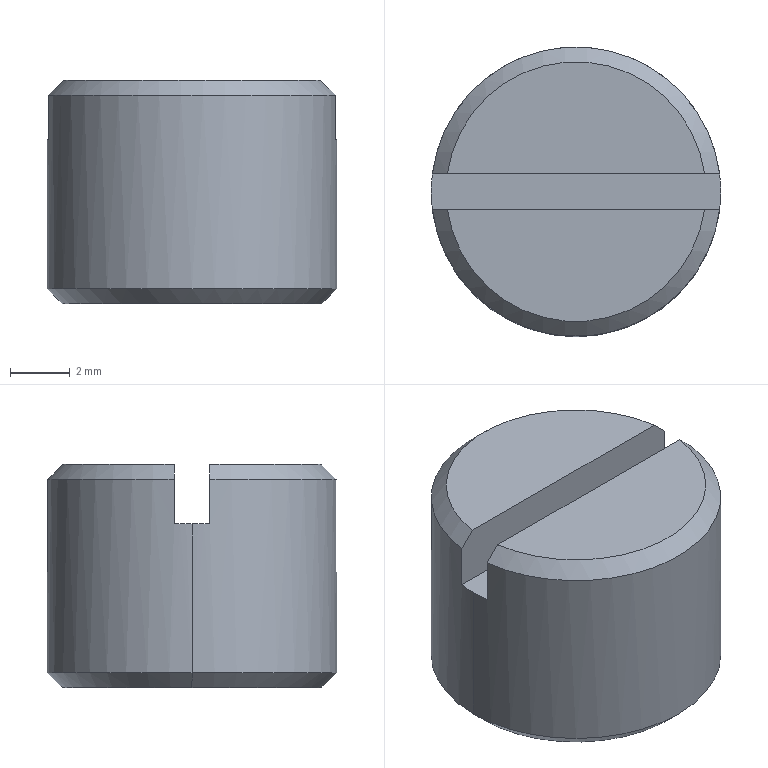Part | SolidWorks | features Chamfer 1, Extrusion 1, ICE 1 | 1 solid | 12 faces | box 9.73 x 9.73 x 7.5 mm | volume 527.297 mm3 | plane 6 | cone 4 | cylinder 2 | commonest cylinder face diameters 9.73 x2
STEP:
#1=CARTESIAN_POINT('',(-4.365,0.,0.));
#2=VERTEX_POINT('',#1);
#3=CARTESIAN_POINT('',(4.365,0.,0.));
#4=VERTEX_POINT('',#3);
#5=CARTESIAN_POINT('',(0.,0.,0.));
#6=DIRECTION('',(0.,0.,-1.));
#7=DIRECTION('',(1.,0.,0.));
#8=AXIS2_PLACEMENT_3D('',#5,#6,#7);
#9=CIRCLE('',#8,4.365);
#10=EDGE_CURVE('',#2,#4,#9,.T.);
#11=ORIENTED_EDGE('',*,*,#10,.F.);
#12=CARTESIAN_POINT('',(-4.865,0.,0.5));
#13=VERTEX_POINT('',#12);
#14=CARTESIAN_POINT('',(-4.865,0.,0.5));
#15=DIRECTION('',(-0.7071,0.,0.7071));
#16=VECTOR('',#15,1000.);
#17=LINE('',#14,#16);
#18=EDGE_CURVE('',#2,#13,#17,.T.);
#19=ORIENTED_EDGE('',*,*,#18,.T.);
#20=CARTESIAN_POINT('',(4.865,0.,0.5));
#21=VERTEX_POINT('',#20);
#22=CARTESIAN_POINT('',(0.,0.,0.5));
#23=DIRECTION('',(0.,0.,1.));
#24=DIRECTION('',(1.,0.,0.));
#25=AXIS2_PLACEMENT_3D('',#22,#23,#24);
#26=CIRCLE('',#25,4.865);
#27=EDGE_CURVE('',#21,#13,#26,.T.);
#28=ORIENTED_EDGE('',*,*,#27,.F.);
#29=CARTESIAN_POINT('',(4.865,0.,0.5));
#30=DIRECTION('',(0.7071,0.,0.7071));
#31=VECTOR('',#30,1000.);
#32=LINE('',#29,#31);
#33=EDGE_CURVE('',#4,#21,#32,.T.);
#34=ORIENTED_EDGE('',*,*,#33,.F.);
#35=EDGE_LOOP('',(#11,#19,#28,#34));
#36=FACE_OUTER_BOUND('',#35,.T.);
#37=CARTESIAN_POINT('',(0.,0.,0.5));
#38=DIRECTION('',(0.,0.,1.));
#39=DIRECTION('',(1.,0.,0.));
#40=AXIS2_PLACEMENT_3D('',#37,#38,#39);
#41=CONICAL_SURFACE('',#40,4.865,0.7854);
#42=ADVANCED_FACE('',(#36),#41,.T.);
#43=CARTESIAN_POINT('',(4.865,0.,5.5));
#44=VERTEX_POINT('',#43);
#45=CARTESIAN_POINT('',(4.828,0.6,5.5));
#46=VERTEX_POINT('',#45);
#47=CARTESIAN_POINT('',(0.,0.,5.5));
#48=DIRECTION('',(0.,0.,1.));
#49=DIRECTION('',(1.,0.,0.));
#50=AXIS2_PLACEMENT_3D('',#47,#48,#49);
#51=CIRCLE('',#50,4.865);
#52=EDGE_CURVE('',#44,#46,#51,.T.);
#53=ORIENTED_EDGE('',*,*,#52,.F.);
#54=CARTESIAN_POINT('',(4.865,0.,7.5));
#55=DIRECTION('',(0.,0.,-1.));
#56=VECTOR('',#55,1000.);
#57=LINE('',#54,#56);
#58=EDGE_CURVE('',#44,#21,#57,.T.);
#59=ORIENTED_EDGE('',*,*,#58,.T.);
#60=ORIENTED_EDGE('',*,*,#27,.T.);
#61=CARTESIAN_POINT('',(-4.865,0.,5.5));
#62=VERTEX_POINT('',#61);
#63=CARTESIAN_POINT('',(-4.865,0.,7.5));
#64=DIRECTION('',(0.,0.,-1.));
#65=VECTOR('',#64,1000.);
#66=LINE('',#63,#65);
#67=EDGE_CURVE('',#62,#13,#66,.T.);
#68=ORIENTED_EDGE('',*,*,#67,.F.);
#69=CARTESIAN_POINT('',(-4.828,0.6,5.5));
#70=VERTEX_POINT('',#69);
#71=CARTESIAN_POINT('',(0.,0.,5.5));
#72=DIRECTION('',(0.,0.,1.));
#73=DIRECTION('',(1.,0.,0.));
#74=AXIS2_PLACEMENT_3D('',#71,#72,#73);
#75=CIRCLE('',#74,4.865);
#76=EDGE_CURVE('',#70,#62,#75,.T.);
#77=ORIENTED_EDGE('',*,*,#76,.F.);
#78=CARTESIAN_POINT('',(-4.828,0.6,7.));
#79=VERTEX_POINT('',#78);
#80=CARTESIAN_POINT('',(-4.828,0.6,7.5));
#81=DIRECTION('',(0.,0.,1.));
#82=VECTOR('',#81,1000.);
#83=LINE('',#80,#82);
#84=EDGE_CURVE('',#70,#79,#83,.T.);
#85=ORIENTED_EDGE('',*,*,#84,.T.);
#86=CARTESIAN_POINT('',(4.828,0.6,7.));
#87=VERTEX_POINT('',#86);
#88=CARTESIAN_POINT('',(0.,0.,7.));
#89=DIRECTION('',(0.,0.,-1.));
#90=DIRECTION('',(1.,0.,0.));
#91=AXIS2_PLACEMENT_3D('',#88,#89,#90);
#92=CIRCLE('',#91,4.865);
#93=EDGE_CURVE('',#79,#87,#92,.T.);
#94=ORIENTED_EDGE('',*,*,#93,.T.);
#95=CARTESIAN_POINT('',(4.828,0.6,7.5));
#96=DIRECTION('',(0.,0.,-1.));
#97=VECTOR('',#96,1000.);
#98=LINE('',#95,#97);
#99=EDGE_CURVE('',#87,#46,#98,.T.);
#100=ORIENTED_EDGE('',*,*,#99,.T.);
#101=EDGE_LOOP('',(#53,#59,#60,#68,#77,#85,#94,#100));
#102=FACE_OUTER_BOUND('',#101,.T.);
#103=CARTESIAN_POINT('',(0.,0.,7.5));
#104=DIRECTION('',(0.,0.,-1.));
#105=DIRECTION('',(-1.,0.,0.));
#106=AXIS2_PLACEMENT_3D('',#103,#104,#105);
#107=CYLINDRICAL_SURFACE('',#106,4.865);
#108=ADVANCED_FACE('',(#102),#107,.T.);
#109=CARTESIAN_POINT('',(4.324,0.6,7.5));
#110=VERTEX_POINT('',#109);
#111=CARTESIAN_POINT('',(-4.324,0.6,7.5));
#112=VERTEX_POINT('',#111);
#113=CARTESIAN_POINT('',(0.,0.6,7.5));
#114=DIRECTION('',(-1.,0.,0.));
#115=VECTOR('',#114,1000.);
#116=LINE('',#113,#115);
#117=EDGE_CURVE('',#110,#112,#116,.T.);
#118=ORIENTED_EDGE('',*,*,#117,.F.);
#119=CARTESIAN_POINT('',(0.,0.,7.5));
#120=DIRECTION('',(0.,0.,1.));
#121=DIRECTION('',(1.,0.,0.));
#122=AXIS2_PLACEMENT_3D('',#119,#120,#121);
#123=CIRCLE('',#122,4.365);
#124=EDGE_CURVE('',#110,#112,#123,.T.);
#125=ORIENTED_EDGE('',*,*,#124,.T.);
#126=EDGE_LOOP('',(#118,#125));
#127=FACE_OUTER_BOUND('',#126,.T.);
#128=CARTESIAN_POINT('',(0.,0.,7.5));
#129=DIRECTION('',(0.,0.,1.));
#130=DIRECTION('',(1.,0.,0.));
#131=AXIS2_PLACEMENT_3D('',#128,#129,#130);
#132=PLANE('',#131);
#133=ADVANCED_FACE('',(#127),#132,.T.);
#134=ORIENTED_EDGE('',*,*,#58,.F.);
#135=CARTESIAN_POINT('',(4.828,-0.6,5.5));
#136=VERTEX_POINT('',#135);
#137=CARTESIAN_POINT('',(0.,0.,5.5));
#138=DIRECTION('',(0.,0.,1.));
#139=DIRECTION('',(1.,0.,0.));
#140=AXIS2_PLACEMENT_3D('',#137,#138,#139);
#141=CIRCLE('',#140,4.865);
#142=EDGE_CURVE('',#136,#44,#141,.T.);
#143=ORIENTED_EDGE('',*,*,#142,.F.);
#144=CARTESIAN_POINT('',(4.828,-0.6,7.));
#145=VERTEX_POINT('',#144);
#146=CARTESIAN_POINT('',(4.828,-0.6,7.5));
#147=DIRECTION('',(0.,0.,1.));
#148=VECTOR('',#147,1000.);
#149=LINE('',#146,#148);
#150=EDGE_CURVE('',#136,#145,#149,.T.);
#151=ORIENTED_EDGE('',*,*,#150,.T.);
#152=CARTESIAN_POINT('',(-4.828,-0.6,7.));
#153=VERTEX_POINT('',#152);
#154=CARTESIAN_POINT('',(0.,0.,7.));
#155=DIRECTION('',(0.,0.,-1.));
#156=DIRECTION('',(1.,0.,0.));
#157=AXIS2_PLACEMENT_3D('',#154,#155,#156);
#158=CIRCLE('',#157,4.865);
#159=EDGE_CURVE('',#145,#153,#158,.T.);
#160=ORIENTED_EDGE('',*,*,#159,.T.);
#161=CARTESIAN_POINT('',(-4.828,-0.6,5.5));
#162=VERTEX_POINT('',#161);
#163=CARTESIAN_POINT('',(-4.828,-0.6,7.5));
#164=DIRECTION('',(0.,0.,-1.));
#165=VECTOR('',#164,1000.);
#166=LINE('',#163,#165);
#167=EDGE_CURVE('',#153,#162,#166,.T.);
#168=ORIENTED_EDGE('',*,*,#167,.T.);
#169=CARTESIAN_POINT('',(0.,0.,5.5));
#170=DIRECTION('',(0.,0.,1.));
#171=DIRECTION('',(1.,0.,0.));
#172=AXIS2_PLACEMENT_3D('',#169,#170,#171);
#173=CIRCLE('',#172,4.865);
#174=EDGE_CURVE('',#62,#162,#173,.T.);
#175=ORIENTED_EDGE('',*,*,#174,.F.);
#176=ORIENTED_EDGE('',*,*,#67,.T.);
#177=CARTESIAN_POINT('',(0.,0.,0.5));
#178=DIRECTION('',(0.,0.,1.));
#179=DIRECTION('',(1.,0.,0.));
#180=AXIS2_PLACEMENT_3D('',#177,#178,#179);
#181=CIRCLE('',#180,4.865);
#182=EDGE_CURVE('',#13,#21,#181,.T.);
#183=ORIENTED_EDGE('',*,*,#182,.T.);
#184=EDGE_LOOP('',(#134,#143,#151,#160,#168,#175,#176,#183));
#185=FACE_OUTER_BOUND('',#184,.T.);
#186=CARTESIAN_POINT('',(0.,0.,7.5));
#187=DIRECTION('',(0.,0.,-1.));
#188=DIRECTION('',(-1.,0.,0.));
#189=AXIS2_PLACEMENT_3D('',#186,#187,#188);
#190=CYLINDRICAL_SURFACE('',#189,4.865);
#191=ADVANCED_FACE('',(#185),#190,.T.);
#192=CARTESIAN_POINT('',(-4.324,-0.6,7.5));
#193=VERTEX_POINT('',#192);
#194=CARTESIAN_POINT('',(4.324,-0.6,7.5));
#195=VERTEX_POINT('',#194);
#196=CARTESIAN_POINT('',(0.,-0.6,7.5));
#197=DIRECTION('',(1.,0.,0.));
#198=VECTOR('',#197,1000.);
#199=LINE('',#196,#198);
#200=EDGE_CURVE('',#193,#195,#199,.T.);
#201=ORIENTED_EDGE('',*,*,#200,.F.);
#202=CARTESIAN_POINT('',(0.,0.,7.5));
#203=DIRECTION('',(0.,0.,1.));
#204=DIRECTION('',(1.,0.,0.));
#205=AXIS2_PLACEMENT_3D('',#202,#203,#204);
#206=CIRCLE('',#205,4.365);
#207=EDGE_CURVE('',#193,#195,#206,.T.);
#208=ORIENTED_EDGE('',*,*,#207,.T.);
#209=EDGE_LOOP('',(#201,#208));
#210=FACE_OUTER_BOUND('',#209,.T.);
#211=CARTESIAN_POINT('',(0.,0.,7.5));
#212=DIRECTION('',(0.,0.,1.));
#213=DIRECTION('',(1.,0.,0.));
#214=AXIS2_PLACEMENT_3D('',#211,#212,#213);
#215=PLANE('',#214);
#216=ADVANCED_FACE('',(#210),#215,.T.);
#217=CARTESIAN_POINT('',(0.,0.,0.));
#218=DIRECTION('',(0.,0.,-1.));
#219=DIRECTION('',(1.,0.,0.));
#220=AXIS2_PLACEMENT_3D('',#217,#218,#219);
#221=CIRCLE('',#220,4.365);
#222=EDGE_CURVE('',#4,#2,#221,.T.);
#223=ORIENTED_EDGE('',*,*,#222,.T.);
#224=ORIENTED_EDGE('',*,*,#10,.T.);
#225=EDGE_LOOP('',(#223,#224));
#226=FACE_OUTER_BOUND('',#225,.T.);
#227=CARTESIAN_POINT('',(0.,0.,0.));
#228=DIRECTION('',(0.,0.,1.));
#229=DIRECTION('',(1.,0.,0.));
#230=AXIS2_PLACEMENT_3D('',#227,#228,#229);
#231=PLANE('',#230);
#232=ADVANCED_FACE('',(#226),#231,.F.);
#233=ORIENTED_EDGE('',*,*,#76,.T.);
#234=ORIENTED_EDGE('',*,*,#174,.T.);
#235=CARTESIAN_POINT('',(6.41,-0.6,5.5));
#236=DIRECTION('',(1.,0.,0.));
#237=VECTOR('',#236,1000.);
#238=LINE('',#235,#237);
#239=EDGE_CURVE('',#162,#136,#238,.T.);
#240=ORIENTED_EDGE('',*,*,#239,.T.);
#241=ORIENTED_EDGE('',*,*,#142,.T.);
#242=ORIENTED_EDGE('',*,*,#52,.T.);
#243=CARTESIAN_POINT('',(6.41,0.6,5.5));
#244=DIRECTION('',(-1.,0.,0.));
#245=VECTOR('',#244,1000.);
#246=LINE('',#243,#245);
#247=EDGE_CURVE('',#46,#70,#246,.T.);
#248=ORIENTED_EDGE('',*,*,#247,.T.);
#249=EDGE_LOOP('',(#233,#234,#240,#241,#242,#248));
#250=FACE_OUTER_BOUND('',#249,.T.);
#251=CARTESIAN_POINT('',(0.,0.,5.5));
#252=DIRECTION('',(0.,0.,1.));
#253=DIRECTION('',(1.,0.,0.));
#254=AXIS2_PLACEMENT_3D('',#251,#252,#253);
#255=PLANE('',#254);
#256=ADVANCED_FACE('',(#250),#255,.T.);
#257=ORIENTED_EDGE('',*,*,#117,.T.);
#258=CARTESIAN_POINT('',(-4.324,0.6,7.5));
#259=CARTESIAN_POINT('',(-4.492,0.6,7.333));
#260=CARTESIAN_POINT('',(-4.66,0.6,7.167));
#261=CARTESIAN_POINT('',(-4.828,0.6,7.));
#262=B_SPLINE_CURVE_WITH_KNOTS('',3,(#258,#259,#260,#261),.UNSPECIFIED.,.F.,.F.,(4,4),(0.,0.0007101),.UNSPECIFIED.);
#263=EDGE_CURVE('',#112,#79,#262,.T.);
#264=ORIENTED_EDGE('',*,*,#263,.T.);
#265=ORIENTED_EDGE('',*,*,#84,.F.);
#266=ORIENTED_EDGE('',*,*,#247,.F.);
#267=ORIENTED_EDGE('',*,*,#99,.F.);
#268=CARTESIAN_POINT('',(4.828,0.6,7.));
#269=CARTESIAN_POINT('',(4.66,0.6,7.167));
#270=CARTESIAN_POINT('',(4.492,0.6,7.333));
#271=CARTESIAN_POINT('',(4.324,0.6,7.5));
#272=B_SPLINE_CURVE_WITH_KNOTS('',3,(#268,#269,#270,#271),.UNSPECIFIED.,.F.,.F.,(4,4),(0.,0.0007101),.UNSPECIFIED.);
#273=EDGE_CURVE('',#87,#110,#272,.T.);
#274=ORIENTED_EDGE('',*,*,#273,.T.);
#275=EDGE_LOOP('',(#257,#264,#265,#266,#267,#274));
#276=FACE_OUTER_BOUND('',#275,.T.);
#277=CARTESIAN_POINT('',(6.41,0.6,5.5));
#278=DIRECTION('',(0.,1.,0.));
#279=DIRECTION('',(-1.,0.,0.));
#280=AXIS2_PLACEMENT_3D('',#277,#278,#279);
#281=PLANE('',#280);
#282=ADVANCED_FACE('',(#276),#281,.F.);
#283=ORIENTED_EDGE('',*,*,#200,.T.);
#284=CARTESIAN_POINT('',(4.324,-0.6,7.5));
#285=CARTESIAN_POINT('',(4.492,-0.6,7.333));
#286=CARTESIAN_POINT('',(4.66,-0.6,7.167));
#287=CARTESIAN_POINT('',(4.828,-0.6,7.));
#288=B_SPLINE_CURVE_WITH_KNOTS('',3,(#284,#285,#286,#287),.UNSPECIFIED.,.F.,.F.,(4,4),(0.,0.0007101),.UNSPECIFIED.);
#289=EDGE_CURVE('',#195,#145,#288,.T.);
#290=ORIENTED_EDGE('',*,*,#289,.T.);
#291=ORIENTED_EDGE('',*,*,#150,.F.);
#292=ORIENTED_EDGE('',*,*,#239,.F.);
#293=ORIENTED_EDGE('',*,*,#167,.F.);
#294=CARTESIAN_POINT('',(-4.828,-0.6,7.));
#295=CARTESIAN_POINT('',(-4.66,-0.6,7.167));
#296=CARTESIAN_POINT('',(-4.492,-0.6,7.333));
#297=CARTESIAN_POINT('',(-4.324,-0.6,7.5));
#298=B_SPLINE_CURVE_WITH_KNOTS('',3,(#294,#295,#296,#297),.UNSPECIFIED.,.F.,.F.,(4,4),(0.,0.0007101),.UNSPECIFIED.);
#299=EDGE_CURVE('',#153,#193,#298,.T.);
#300=ORIENTED_EDGE('',*,*,#299,.T.);
#301=EDGE_LOOP('',(#283,#290,#291,#292,#293,#300));
#302=FACE_OUTER_BOUND('',#301,.T.);
#303=CARTESIAN_POINT('',(6.41,-0.6,5.5));
#304=DIRECTION('',(0.,-1.,0.));
#305=DIRECTION('',(1.,0.,0.));
#306=AXIS2_PLACEMENT_3D('',#303,#304,#305);
#307=PLANE('',#306);
#308=ADVANCED_FACE('',(#302),#307,.F.);
#309=ORIENTED_EDGE('',*,*,#18,.F.);
#310=ORIENTED_EDGE('',*,*,#222,.F.);
#311=ORIENTED_EDGE('',*,*,#33,.T.);
#312=ORIENTED_EDGE('',*,*,#182,.F.);
#313=EDGE_LOOP('',(#309,#310,#311,#312));
#314=FACE_OUTER_BOUND('',#313,.T.);
#315=CARTESIAN_POINT('',(0.,0.,0.5));
#316=DIRECTION('',(0.,0.,1.));
#317=DIRECTION('',(1.,0.,0.));
#318=AXIS2_PLACEMENT_3D('',#315,#316,#317);
#319=CONICAL_SURFACE('',#318,4.865,0.7854);
#320=ADVANCED_FACE('',(#314),#319,.T.);
#321=ORIENTED_EDGE('',*,*,#299,.F.);
#322=ORIENTED_EDGE('',*,*,#159,.F.);
#323=ORIENTED_EDGE('',*,*,#289,.F.);
#324=ORIENTED_EDGE('',*,*,#207,.F.);
#325=EDGE_LOOP('',(#321,#322,#323,#324));
#326=FACE_OUTER_BOUND('',#325,.T.);
#327=CARTESIAN_POINT('',(0.,0.,7.5));
#328=DIRECTION('',(0.,0.,-1.));
#329=DIRECTION('',(-1.,0.,0.));
#330=AXIS2_PLACEMENT_3D('',#327,#328,#329);
#331=CONICAL_SURFACE('',#330,4.365,0.7854);
#332=ADVANCED_FACE('',(#326),#331,.T.);
#333=ORIENTED_EDGE('',*,*,#273,.F.);
#334=ORIENTED_EDGE('',*,*,#93,.F.);
#335=ORIENTED_EDGE('',*,*,#263,.F.);
#336=ORIENTED_EDGE('',*,*,#124,.F.);
#337=EDGE_LOOP('',(#333,#334,#335,#336));
#338=FACE_OUTER_BOUND('',#337,.T.);
#339=CARTESIAN_POINT('',(0.,0.,7.5));
#340=DIRECTION('',(0.,0.,-1.));
#341=DIRECTION('',(-1.,0.,0.));
#342=AXIS2_PLACEMENT_3D('',#339,#340,#341);
#343=CONICAL_SURFACE('',#342,4.365,0.7854);
#344=ADVANCED_FACE('',(#338),#343,.T.);
#345=CLOSED_SHELL('',(#42,#108,#133,#191,#216,#232,#256,#282,#308,#320,#332,#344));
#346=MANIFOLD_SOLID_BREP('',#345);
#347=CARTESIAN_POINT('',(0.,0.,0.));
#348=DIRECTION('',(0.,0.,1.));
#349=DIRECTION('',(1.,0.,0.));
#350=AXIS2_PLACEMENT_3D('',#347,#348,#349);
#351=(LENGTH_UNIT()NAMED_UNIT(*)SI_UNIT(.MILLI.,.METRE.));
#352=UNCERTAINTY_MEASURE_WITH_UNIT(LENGTH_MEASURE(0.00001),#351,'','');
#353=(NAMED_UNIT(*)PLANE_ANGLE_UNIT()SI_UNIT($,.RADIAN.));
#354=(NAMED_UNIT(*)SI_UNIT($,.STERADIAN.)SOLID_ANGLE_UNIT());
#355=(GEOMETRIC_REPRESENTATION_CONTEXT(3)GLOBAL_UNCERTAINTY_ASSIGNED_CONTEXT((#352))GLOBAL_UNIT_ASSIGNED_CONTEXT((#351,#353,#354))REPRESENTATION_CONTEXT('',''));
#356=ADVANCED_BREP_SHAPE_REPRESENTATION('',(#346,#350),#355);